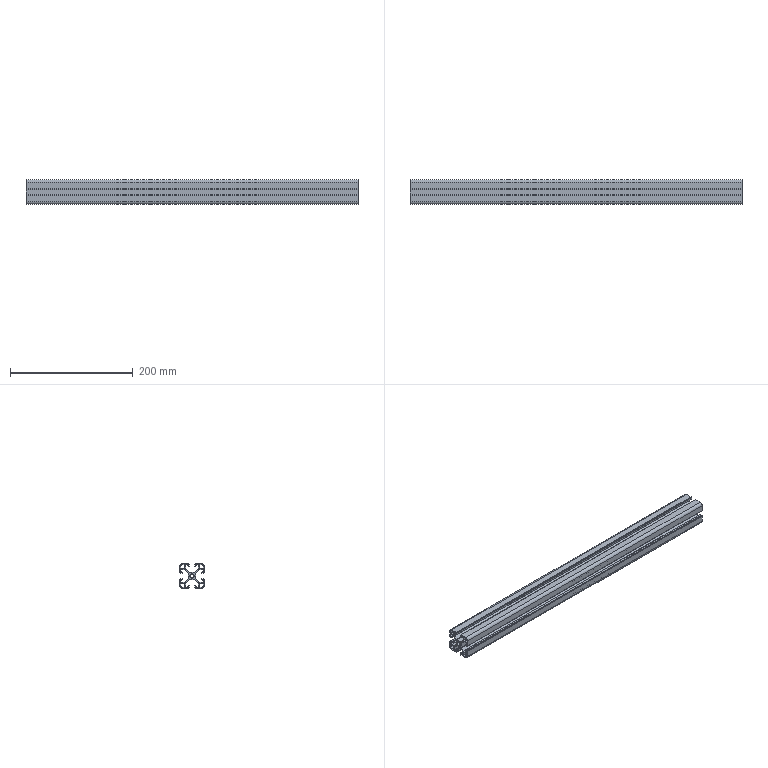Part | STEP file | MK-8-4040C-L-00 profile 4040C standard type 540mm | 1 solid | 188 faces | box 540 x 40 x 40 mm | volume 258254 mm3 | cylinder 94 | plane 94 | commonest cylinder face diameters 0.6 x30 2 x28 4 x16 0.4 x8 6 x4 9 x4